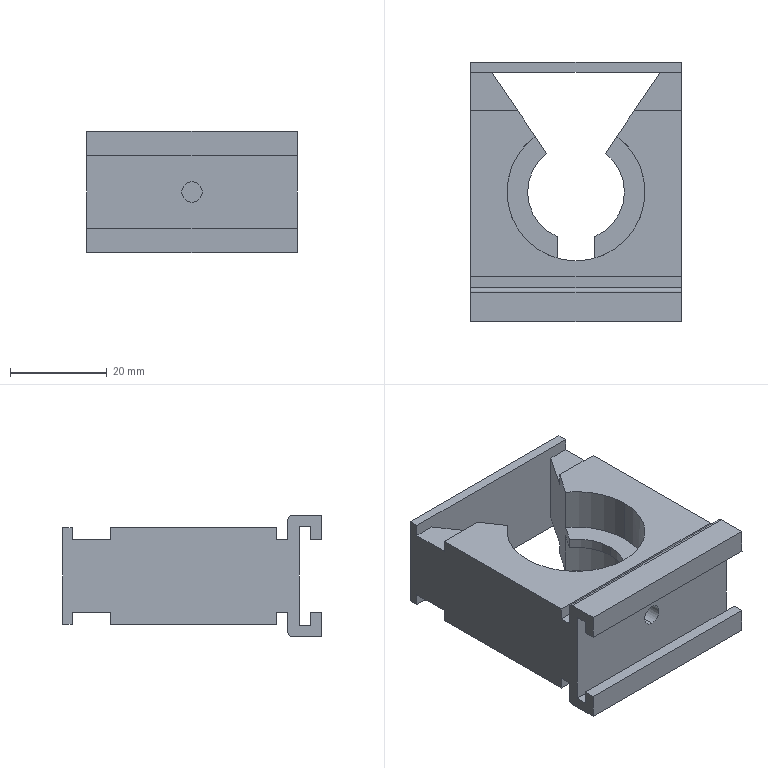Part | STEP file | 00192290_EZT_KLEMMSCHELLE_MKRS-23-B.2 | 1 solid | 55 faces | box 43.5 x 53.5 x 25 mm | volume 24720 mm3 | plane 40 | cylinder 15 | commonest cylinder face diameters 28.5 x6 20 x3 2 x2 4.2 x2 8 x2